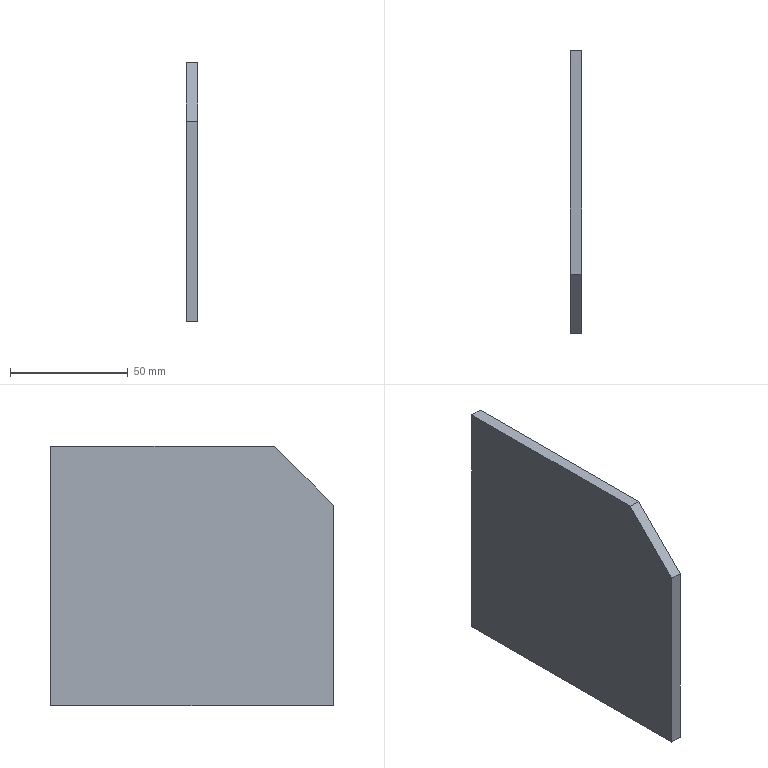Part | SolidWorks | features BaseBody 1 | 1 solid | 7 faces | box 5 x 120 x 110 mm | volume 64438 mm3 | plane 7
STEP:
#1=CARTESIAN_POINT('',(-66.253,569.,-437.5));
#2=VERTEX_POINT('',#1);
#3=CARTESIAN_POINT('',(-66.253,569.,-327.5));
#4=VERTEX_POINT('',#3);
#5=CARTESIAN_POINT('',(-66.253,569.,-442.5));
#6=DIRECTION('',(0.,0.,1.));
#7=VECTOR('',#6,1000.);
#8=LINE('',#5,#7);
#9=EDGE_CURVE('',#2,#4,#8,.T.);
#10=ORIENTED_EDGE('',*,*,#9,.T.);
#11=CARTESIAN_POINT('',(-66.253,474.,-327.5));
#12=VERTEX_POINT('',#11);
#13=CARTESIAN_POINT('',(-66.253,429.,-327.5));
#14=DIRECTION('',(0.,-1.,0.));
#15=VECTOR('',#14,1000.);
#16=LINE('',#13,#15);
#17=EDGE_CURVE('',#4,#12,#16,.T.);
#18=ORIENTED_EDGE('',*,*,#17,.T.);
#19=CARTESIAN_POINT('',(-66.253,449.,-352.5));
#20=VERTEX_POINT('',#19);
#21=CARTESIAN_POINT('',(-66.253,474.,-327.5));
#22=DIRECTION('',(0.,-0.7071,-0.7071));
#23=VECTOR('',#22,1000.);
#24=LINE('',#21,#23);
#25=EDGE_CURVE('',#12,#20,#24,.T.);
#26=ORIENTED_EDGE('',*,*,#25,.T.);
#27=CARTESIAN_POINT('',(-66.253,449.,-437.5));
#28=VERTEX_POINT('',#27);
#29=CARTESIAN_POINT('',(-66.253,449.,-442.5));
#30=DIRECTION('',(0.,0.,-1.));
#31=VECTOR('',#30,1000.);
#32=LINE('',#29,#31);
#33=EDGE_CURVE('',#20,#28,#32,.T.);
#34=ORIENTED_EDGE('',*,*,#33,.T.);
#35=CARTESIAN_POINT('',(-66.253,429.,-437.5));
#36=DIRECTION('',(0.,1.,0.));
#37=VECTOR('',#36,1000.);
#38=LINE('',#35,#37);
#39=EDGE_CURVE('',#28,#2,#38,.T.);
#40=ORIENTED_EDGE('',*,*,#39,.T.);
#41=EDGE_LOOP('',(#10,#18,#26,#34,#40));
#42=FACE_OUTER_BOUND('',#41,.T.);
#43=CARTESIAN_POINT('',(-66.253,429.,-442.5));
#44=DIRECTION('',(1.,0.,0.));
#45=DIRECTION('',(0.,0.,-1.));
#46=AXIS2_PLACEMENT_3D('',#43,#44,#45);
#47=PLANE('',#46);
#48=ADVANCED_FACE('',(#42),#47,.T.);
#49=ORIENTED_EDGE('',*,*,#17,.F.);
#50=CARTESIAN_POINT('',(-71.253,569.,-327.5));
#51=VERTEX_POINT('',#50);
#52=CARTESIAN_POINT('',(-66.253,569.,-327.5));
#53=DIRECTION('',(1.,0.,0.));
#54=VECTOR('',#53,1000.);
#55=LINE('',#52,#54);
#56=EDGE_CURVE('',#51,#4,#55,.T.);
#57=ORIENTED_EDGE('',*,*,#56,.F.);
#58=CARTESIAN_POINT('',(-71.253,474.,-327.5));
#59=VERTEX_POINT('',#58);
#60=CARTESIAN_POINT('',(-71.253,449.,-327.5));
#61=DIRECTION('',(0.,1.,0.));
#62=VECTOR('',#61,1000.);
#63=LINE('',#60,#62);
#64=EDGE_CURVE('',#59,#51,#63,.T.);
#65=ORIENTED_EDGE('',*,*,#64,.F.);
#66=CARTESIAN_POINT('',(-66.253,474.,-327.5));
#67=DIRECTION('',(-1.,0.,0.));
#68=VECTOR('',#67,1000.);
#69=LINE('',#66,#68);
#70=EDGE_CURVE('',#12,#59,#69,.T.);
#71=ORIENTED_EDGE('',*,*,#70,.F.);
#72=EDGE_LOOP('',(#49,#57,#65,#71));
#73=FACE_OUTER_BOUND('',#72,.T.);
#74=CARTESIAN_POINT('',(-66.253,449.,-327.5));
#75=DIRECTION('',(0.,0.,-1.));
#76=DIRECTION('',(-1.,0.,0.));
#77=AXIS2_PLACEMENT_3D('',#74,#75,#76);
#78=PLANE('',#77);
#79=ADVANCED_FACE('',(#73),#78,.F.);
#80=ORIENTED_EDGE('',*,*,#9,.F.);
#81=CARTESIAN_POINT('',(-71.253,569.,-437.5));
#82=VERTEX_POINT('',#81);
#83=CARTESIAN_POINT('',(-66.253,569.,-437.5));
#84=DIRECTION('',(1.,0.,0.));
#85=VECTOR('',#84,1000.);
#86=LINE('',#83,#85);
#87=EDGE_CURVE('',#82,#2,#86,.T.);
#88=ORIENTED_EDGE('',*,*,#87,.F.);
#89=CARTESIAN_POINT('',(-71.253,569.,-437.5));
#90=DIRECTION('',(0.,0.,-1.));
#91=VECTOR('',#90,1000.);
#92=LINE('',#89,#91);
#93=EDGE_CURVE('',#51,#82,#92,.T.);
#94=ORIENTED_EDGE('',*,*,#93,.F.);
#95=ORIENTED_EDGE('',*,*,#56,.T.);
#96=EDGE_LOOP('',(#80,#88,#94,#95));
#97=FACE_OUTER_BOUND('',#96,.T.);
#98=CARTESIAN_POINT('',(-66.253,569.,-437.5));
#99=DIRECTION('',(0.,-1.,0.));
#100=DIRECTION('',(0.,0.,-1.));
#101=AXIS2_PLACEMENT_3D('',#98,#99,#100);
#102=PLANE('',#101);
#103=ADVANCED_FACE('',(#97),#102,.F.);
#104=ORIENTED_EDGE('',*,*,#39,.F.);
#105=CARTESIAN_POINT('',(-71.253,449.,-437.5));
#106=VERTEX_POINT('',#105);
#107=CARTESIAN_POINT('',(-66.253,449.,-437.5));
#108=DIRECTION('',(1.,0.,0.));
#109=VECTOR('',#108,1000.);
#110=LINE('',#107,#109);
#111=EDGE_CURVE('',#106,#28,#110,.T.);
#112=ORIENTED_EDGE('',*,*,#111,.F.);
#113=CARTESIAN_POINT('',(-71.253,449.,-437.5));
#114=DIRECTION('',(0.,-1.,0.));
#115=VECTOR('',#114,1000.);
#116=LINE('',#113,#115);
#117=EDGE_CURVE('',#82,#106,#116,.T.);
#118=ORIENTED_EDGE('',*,*,#117,.F.);
#119=ORIENTED_EDGE('',*,*,#87,.T.);
#120=EDGE_LOOP('',(#104,#112,#118,#119));
#121=FACE_OUTER_BOUND('',#120,.T.);
#122=CARTESIAN_POINT('',(-66.253,449.,-437.5));
#123=DIRECTION('',(0.,0.,1.));
#124=DIRECTION('',(1.,0.,0.));
#125=AXIS2_PLACEMENT_3D('',#122,#123,#124);
#126=PLANE('',#125);
#127=ADVANCED_FACE('',(#121),#126,.F.);
#128=CARTESIAN_POINT('',(-71.253,449.,-352.5));
#129=VERTEX_POINT('',#128);
#130=CARTESIAN_POINT('',(-71.253,449.,-437.5));
#131=DIRECTION('',(0.,0.,1.));
#132=VECTOR('',#131,1000.);
#133=LINE('',#130,#132);
#134=EDGE_CURVE('',#106,#129,#133,.T.);
#135=ORIENTED_EDGE('',*,*,#134,.F.);
#136=ORIENTED_EDGE('',*,*,#111,.T.);
#137=ORIENTED_EDGE('',*,*,#33,.F.);
#138=CARTESIAN_POINT('',(-66.253,449.,-352.5));
#139=DIRECTION('',(1.,0.,0.));
#140=VECTOR('',#139,1000.);
#141=LINE('',#138,#140);
#142=EDGE_CURVE('',#129,#20,#141,.T.);
#143=ORIENTED_EDGE('',*,*,#142,.F.);
#144=EDGE_LOOP('',(#135,#136,#137,#143));
#145=FACE_OUTER_BOUND('',#144,.T.);
#146=CARTESIAN_POINT('',(-66.253,449.,-437.5));
#147=DIRECTION('',(0.,1.,0.));
#148=DIRECTION('',(0.,0.,1.));
#149=AXIS2_PLACEMENT_3D('',#146,#147,#148);
#150=PLANE('',#149);
#151=ADVANCED_FACE('',(#145),#150,.F.);
#152=CARTESIAN_POINT('',(-71.253,449.,-352.5));
#153=DIRECTION('',(0.,0.7071,0.7071));
#154=VECTOR('',#153,1000.);
#155=LINE('',#152,#154);
#156=EDGE_CURVE('',#129,#59,#155,.T.);
#157=ORIENTED_EDGE('',*,*,#156,.F.);
#158=ORIENTED_EDGE('',*,*,#142,.T.);
#159=ORIENTED_EDGE('',*,*,#25,.F.);
#160=ORIENTED_EDGE('',*,*,#70,.T.);
#161=EDGE_LOOP('',(#157,#158,#159,#160));
#162=FACE_OUTER_BOUND('',#161,.T.);
#163=CARTESIAN_POINT('',(-66.253,449.,-352.5));
#164=DIRECTION('',(0.,0.7071,-0.7071));
#165=DIRECTION('',(0.,0.7071,0.7071));
#166=AXIS2_PLACEMENT_3D('',#163,#164,#165);
#167=PLANE('',#166);
#168=ADVANCED_FACE('',(#162),#167,.F.);
#169=ORIENTED_EDGE('',*,*,#64,.T.);
#170=ORIENTED_EDGE('',*,*,#93,.T.);
#171=ORIENTED_EDGE('',*,*,#117,.T.);
#172=ORIENTED_EDGE('',*,*,#134,.T.);
#173=ORIENTED_EDGE('',*,*,#156,.T.);
#174=EDGE_LOOP('',(#169,#170,#171,#172,#173));
#175=FACE_OUTER_BOUND('',#174,.T.);
#176=CARTESIAN_POINT('',(-71.253,429.,-442.5));
#177=DIRECTION('',(1.,0.,0.));
#178=DIRECTION('',(0.,0.,-1.));
#179=AXIS2_PLACEMENT_3D('',#176,#177,#178);
#180=PLANE('',#179);
#181=ADVANCED_FACE('',(#175),#180,.F.);
#182=CLOSED_SHELL('',(#48,#79,#103,#127,#151,#168,#181));
#183=MANIFOLD_SOLID_BREP('',#182);
#184=CARTESIAN_POINT('',(0.,0.,0.));
#185=DIRECTION('',(0.,0.,1.));
#186=DIRECTION('',(1.,0.,0.));
#187=AXIS2_PLACEMENT_3D('',#184,#185,#186);
#188=(LENGTH_UNIT()NAMED_UNIT(*)SI_UNIT(.MILLI.,.METRE.));
#189=UNCERTAINTY_MEASURE_WITH_UNIT(LENGTH_MEASURE(0.00001),#188,'','');
#190=(NAMED_UNIT(*)PLANE_ANGLE_UNIT()SI_UNIT($,.RADIAN.));
#191=(NAMED_UNIT(*)SI_UNIT($,.STERADIAN.)SOLID_ANGLE_UNIT());
#192=(GEOMETRIC_REPRESENTATION_CONTEXT(3)GLOBAL_UNCERTAINTY_ASSIGNED_CONTEXT((#189))GLOBAL_UNIT_ASSIGNED_CONTEXT((#188,#190,#191))REPRESENTATION_CONTEXT('',''));
#193=ADVANCED_BREP_SHAPE_REPRESENTATION('',(#183,#187),#192);